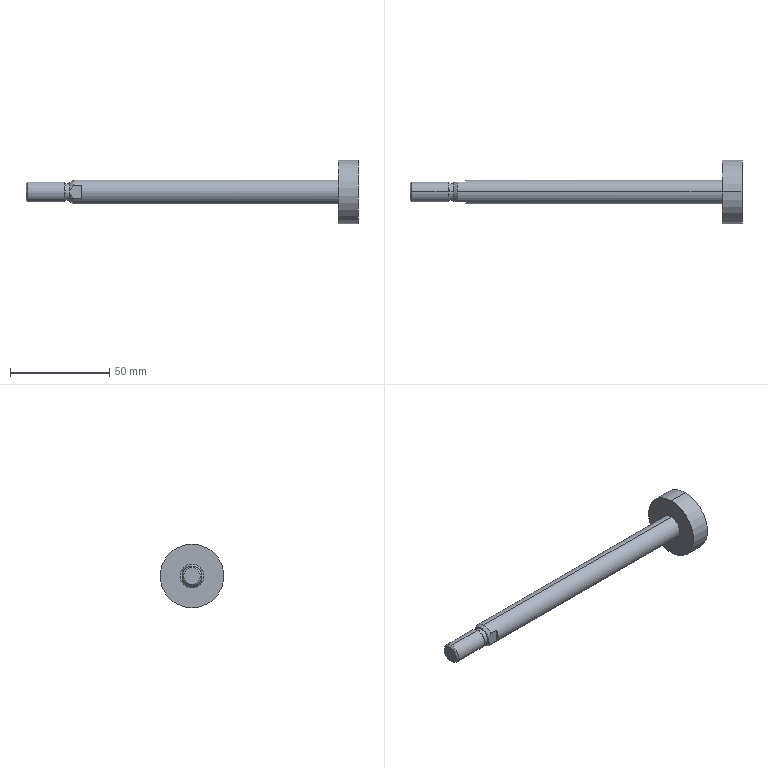Part | SolidWorks | features BaseBody 1 | 1 solid | 23 faces | box 166.9 x 32 x 32 mm | volume 24888 mm3 | plane 9 | cylinder 8 | cone 6 | commonest cylinder face diameters 8.4 x2 10 x2 12 x2 32 x2
STEP:
#1=CARTESIAN_POINT('',(-24.268,5.,3.317));
#2=VERTEX_POINT('',#1);
#3=CARTESIAN_POINT('',(-24.268,0.,6.));
#4=VERTEX_POINT('',#3);
#5=CARTESIAN_POINT('',(-24.268,0.,0.));
#6=DIRECTION('',(1.,0.,0.));
#7=DIRECTION('',(0.,0.,-1.));
#8=AXIS2_PLACEMENT_3D('',#5,#6,#7);
#9=CIRCLE('',#8,6.);
#10=EDGE_CURVE('',#2,#4,#9,.T.);
#11=ORIENTED_EDGE('',*,*,#10,.T.);
#12=CARTESIAN_POINT('',(108.9,0.,6.));
#13=VERTEX_POINT('',#12);
#14=CARTESIAN_POINT('',(118.9,0.,6.));
#15=DIRECTION('',(1.,0.,0.));
#16=VECTOR('',#15,1000.);
#17=LINE('',#14,#16);
#18=EDGE_CURVE('',#4,#13,#17,.T.);
#19=ORIENTED_EDGE('',*,*,#18,.T.);
#20=CARTESIAN_POINT('',(108.9,0.,-6.));
#21=VERTEX_POINT('',#20);
#22=CARTESIAN_POINT('',(108.9,0.,0.));
#23=DIRECTION('',(-1.,0.,0.));
#24=DIRECTION('',(0.,0.,-1.));
#25=AXIS2_PLACEMENT_3D('',#22,#23,#24);
#26=CIRCLE('',#25,6.);
#27=EDGE_CURVE('',#13,#21,#26,.T.);
#28=ORIENTED_EDGE('',*,*,#27,.T.);
#29=CARTESIAN_POINT('',(-24.268,0.,-6.));
#30=VERTEX_POINT('',#29);
#31=CARTESIAN_POINT('',(118.9,0.,-6.));
#32=DIRECTION('',(1.,0.,0.));
#33=VECTOR('',#32,1000.);
#34=LINE('',#31,#33);
#35=EDGE_CURVE('',#30,#21,#34,.T.);
#36=ORIENTED_EDGE('',*,*,#35,.F.);
#37=CARTESIAN_POINT('',(-24.268,5.,-3.317));
#38=VERTEX_POINT('',#37);
#39=CARTESIAN_POINT('',(-24.268,0.,0.));
#40=DIRECTION('',(1.,0.,0.));
#41=DIRECTION('',(0.,0.,-1.));
#42=AXIS2_PLACEMENT_3D('',#39,#40,#41);
#43=CIRCLE('',#42,6.);
#44=EDGE_CURVE('',#30,#38,#43,.T.);
#45=ORIENTED_EDGE('',*,*,#44,.T.);
#46=CARTESIAN_POINT('',(-20.,5.,-3.317));
#47=VERTEX_POINT('',#46);
#48=CARTESIAN_POINT('',(118.9,5.,-3.317));
#49=DIRECTION('',(1.,0.,0.));
#50=VECTOR('',#49,1000.);
#51=LINE('',#48,#50);
#52=EDGE_CURVE('',#38,#47,#51,.T.);
#53=ORIENTED_EDGE('',*,*,#52,.T.);
#54=CARTESIAN_POINT('',(-20.,5.,3.317));
#55=VERTEX_POINT('',#54);
#56=CARTESIAN_POINT('',(-20.,0.,0.));
#57=DIRECTION('',(1.,0.,0.));
#58=DIRECTION('',(0.,0.,-1.));
#59=AXIS2_PLACEMENT_3D('',#56,#57,#58);
#60=CIRCLE('',#59,6.);
#61=EDGE_CURVE('',#47,#55,#60,.T.);
#62=ORIENTED_EDGE('',*,*,#61,.T.);
#63=CARTESIAN_POINT('',(118.9,5.,3.317));
#64=DIRECTION('',(-1.,0.,0.));
#65=VECTOR('',#64,1000.);
#66=LINE('',#63,#65);
#67=EDGE_CURVE('',#55,#2,#66,.T.);
#68=ORIENTED_EDGE('',*,*,#67,.T.);
#69=EDGE_LOOP('',(#11,#19,#28,#36,#45,#53,#62,#68));
#70=FACE_OUTER_BOUND('',#69,.T.);
#71=CARTESIAN_POINT('',(118.9,0.,0.));
#72=DIRECTION('',(1.,0.,0.));
#73=DIRECTION('',(0.,0.,-1.));
#74=AXIS2_PLACEMENT_3D('',#71,#72,#73);
#75=CYLINDRICAL_SURFACE('',#74,6.);
#76=ADVANCED_FACE('',(#70),#75,.T.);
#77=CARTESIAN_POINT('',(108.9,0.,-16.));
#78=VERTEX_POINT('',#77);
#79=CARTESIAN_POINT('',(108.9,0.,16.));
#80=VERTEX_POINT('',#79);
#81=CARTESIAN_POINT('',(108.9,0.,0.));
#82=DIRECTION('',(1.,0.,0.));
#83=DIRECTION('',(0.,0.,-1.));
#84=AXIS2_PLACEMENT_3D('',#81,#82,#83);
#85=CIRCLE('',#84,16.);
#86=EDGE_CURVE('',#78,#80,#85,.T.);
#87=ORIENTED_EDGE('',*,*,#86,.T.);
#88=CARTESIAN_POINT('',(118.9,0.,16.));
#89=VERTEX_POINT('',#88);
#90=CARTESIAN_POINT('',(118.9,0.,16.));
#91=DIRECTION('',(1.,0.,0.));
#92=VECTOR('',#91,1000.);
#93=LINE('',#90,#92);
#94=EDGE_CURVE('',#80,#89,#93,.T.);
#95=ORIENTED_EDGE('',*,*,#94,.T.);
#96=CARTESIAN_POINT('',(118.9,0.,-16.));
#97=VERTEX_POINT('',#96);
#98=CARTESIAN_POINT('',(118.9,0.,0.));
#99=DIRECTION('',(-1.,0.,0.));
#100=DIRECTION('',(0.,0.,-1.));
#101=AXIS2_PLACEMENT_3D('',#98,#99,#100);
#102=CIRCLE('',#101,16.);
#103=EDGE_CURVE('',#89,#97,#102,.T.);
#104=ORIENTED_EDGE('',*,*,#103,.T.);
#105=CARTESIAN_POINT('',(118.9,0.,-16.));
#106=DIRECTION('',(1.,0.,0.));
#107=VECTOR('',#106,1000.);
#108=LINE('',#105,#107);
#109=EDGE_CURVE('',#78,#97,#108,.T.);
#110=ORIENTED_EDGE('',*,*,#109,.F.);
#111=EDGE_LOOP('',(#87,#95,#104,#110));
#112=FACE_OUTER_BOUND('',#111,.T.);
#113=CARTESIAN_POINT('',(118.9,0.,0.));
#114=DIRECTION('',(1.,0.,0.));
#115=DIRECTION('',(0.,0.,-1.));
#116=AXIS2_PLACEMENT_3D('',#113,#114,#115);
#117=CYLINDRICAL_SURFACE('',#116,16.);
#118=ADVANCED_FACE('',(#112),#117,.T.);
#119=CARTESIAN_POINT('',(-28.,0.,-4.2));
#120=VERTEX_POINT('',#119);
#121=CARTESIAN_POINT('',(-28.,0.,4.2));
#122=VERTEX_POINT('',#121);
#123=CARTESIAN_POINT('',(-28.,0.,0.));
#124=DIRECTION('',(1.,0.,0.));
#125=DIRECTION('',(0.,0.,-1.));
#126=AXIS2_PLACEMENT_3D('',#123,#124,#125);
#127=CIRCLE('',#126,4.2);
#128=EDGE_CURVE('',#120,#122,#127,.T.);
#129=ORIENTED_EDGE('',*,*,#128,.T.);
#130=CARTESIAN_POINT('',(-26.,0.,4.2));
#131=VERTEX_POINT('',#130);
#132=CARTESIAN_POINT('',(118.9,0.,4.2));
#133=DIRECTION('',(1.,0.,0.));
#134=VECTOR('',#133,1000.);
#135=LINE('',#132,#134);
#136=EDGE_CURVE('',#122,#131,#135,.T.);
#137=ORIENTED_EDGE('',*,*,#136,.T.);
#138=CARTESIAN_POINT('',(-26.,0.,-4.2));
#139=VERTEX_POINT('',#138);
#140=CARTESIAN_POINT('',(-26.,0.,0.));
#141=DIRECTION('',(-1.,0.,0.));
#142=DIRECTION('',(0.,0.,-1.));
#143=AXIS2_PLACEMENT_3D('',#140,#141,#142);
#144=CIRCLE('',#143,4.2);
#145=EDGE_CURVE('',#131,#139,#144,.T.);
#146=ORIENTED_EDGE('',*,*,#145,.T.);
#147=CARTESIAN_POINT('',(118.9,0.,-4.2));
#148=DIRECTION('',(1.,0.,0.));
#149=VECTOR('',#148,1000.);
#150=LINE('',#147,#149);
#151=EDGE_CURVE('',#120,#139,#150,.T.);
#152=ORIENTED_EDGE('',*,*,#151,.F.);
#153=EDGE_LOOP('',(#129,#137,#146,#152));
#154=FACE_OUTER_BOUND('',#153,.T.);
#155=CARTESIAN_POINT('',(118.9,0.,0.));
#156=DIRECTION('',(1.,0.,0.));
#157=DIRECTION('',(0.,0.,-1.));
#158=AXIS2_PLACEMENT_3D('',#155,#156,#157);
#159=CYLINDRICAL_SURFACE('',#158,4.2);
#160=ADVANCED_FACE('',(#154),#159,.T.);
#161=CARTESIAN_POINT('',(-28.,0.,4.233));
#162=VERTEX_POINT('',#161);
#163=CARTESIAN_POINT('',(-28.,0.,-4.233));
#164=VERTEX_POINT('',#163);
#165=CARTESIAN_POINT('',(-28.,0.,0.));
#166=DIRECTION('',(-1.,0.,0.));
#167=DIRECTION('',(0.,0.,1.));
#168=AXIS2_PLACEMENT_3D('',#165,#166,#167);
#169=CIRCLE('',#168,4.233);
#170=EDGE_CURVE('',#162,#164,#169,.T.);
#171=ORIENTED_EDGE('',*,*,#170,.T.);
#172=CARTESIAN_POINT('',(-28.767,0.,-5.));
#173=VERTEX_POINT('',#172);
#174=CARTESIAN_POINT('',(-28.767,0.,-5.));
#175=DIRECTION('',(-0.7071,0.,-0.7071));
#176=VECTOR('',#175,1000.);
#177=LINE('',#174,#176);
#178=EDGE_CURVE('',#164,#173,#177,.T.);
#179=ORIENTED_EDGE('',*,*,#178,.T.);
#180=CARTESIAN_POINT('',(-28.767,0.,5.));
#181=VERTEX_POINT('',#180);
#182=CARTESIAN_POINT('',(-28.767,0.,0.));
#183=DIRECTION('',(1.,0.,0.));
#184=DIRECTION('',(0.,0.,1.));
#185=AXIS2_PLACEMENT_3D('',#182,#183,#184);
#186=CIRCLE('',#185,5.);
#187=EDGE_CURVE('',#173,#181,#186,.T.);
#188=ORIENTED_EDGE('',*,*,#187,.T.);
#189=CARTESIAN_POINT('',(-28.767,0.,5.));
#190=DIRECTION('',(-0.7071,0.,0.7071));
#191=VECTOR('',#190,1000.);
#192=LINE('',#189,#191);
#193=EDGE_CURVE('',#162,#181,#192,.T.);
#194=ORIENTED_EDGE('',*,*,#193,.F.);
#195=EDGE_LOOP('',(#171,#179,#188,#194));
#196=FACE_OUTER_BOUND('',#195,.T.);
#197=CARTESIAN_POINT('',(-28.767,0.,0.));
#198=DIRECTION('',(-1.,0.,0.));
#199=DIRECTION('',(0.,0.,1.));
#200=AXIS2_PLACEMENT_3D('',#197,#198,#199);
#201=CONICAL_SURFACE('',#200,5.,0.7854);
#202=ADVANCED_FACE('',(#196),#201,.T.);
#203=CARTESIAN_POINT('',(-47.233,0.,-5.));
#204=VERTEX_POINT('',#203);
#205=CARTESIAN_POINT('',(-47.233,0.,5.));
#206=VERTEX_POINT('',#205);
#207=CARTESIAN_POINT('',(-47.233,0.,0.));
#208=DIRECTION('',(1.,0.,0.));
#209=DIRECTION('',(0.,0.,-1.));
#210=AXIS2_PLACEMENT_3D('',#207,#208,#209);
#211=CIRCLE('',#210,5.);
#212=EDGE_CURVE('',#204,#206,#211,.T.);
#213=ORIENTED_EDGE('',*,*,#212,.T.);
#214=CARTESIAN_POINT('',(118.9,0.,5.));
#215=DIRECTION('',(1.,0.,0.));
#216=VECTOR('',#215,1000.);
#217=LINE('',#214,#216);
#218=EDGE_CURVE('',#206,#181,#217,.T.);
#219=ORIENTED_EDGE('',*,*,#218,.T.);
#220=ORIENTED_EDGE('',*,*,#187,.F.);
#221=CARTESIAN_POINT('',(118.9,0.,-5.));
#222=DIRECTION('',(1.,0.,0.));
#223=VECTOR('',#222,1000.);
#224=LINE('',#221,#223);
#225=EDGE_CURVE('',#204,#173,#224,.T.);
#226=ORIENTED_EDGE('',*,*,#225,.F.);
#227=EDGE_LOOP('',(#213,#219,#220,#226));
#228=FACE_OUTER_BOUND('',#227,.T.);
#229=CARTESIAN_POINT('',(118.9,0.,0.));
#230=DIRECTION('',(1.,0.,0.));
#231=DIRECTION('',(0.,0.,-1.));
#232=AXIS2_PLACEMENT_3D('',#229,#230,#231);
#233=CYLINDRICAL_SURFACE('',#232,5.);
#234=ADVANCED_FACE('',(#228),#233,.T.);
#235=CARTESIAN_POINT('',(-48.,0.,-4.233));
#236=VERTEX_POINT('',#235);
#237=CARTESIAN_POINT('',(-48.,0.,4.233));
#238=VERTEX_POINT('',#237);
#239=CARTESIAN_POINT('',(-48.,0.,0.));
#240=DIRECTION('',(1.,0.,0.));
#241=DIRECTION('',(0.,0.,-1.));
#242=AXIS2_PLACEMENT_3D('',#239,#240,#241);
#243=CIRCLE('',#242,4.233);
#244=EDGE_CURVE('',#236,#238,#243,.T.);
#245=ORIENTED_EDGE('',*,*,#244,.T.);
#246=CARTESIAN_POINT('',(-47.233,0.,5.));
#247=DIRECTION('',(0.7071,0.,0.7071));
#248=VECTOR('',#247,1000.);
#249=LINE('',#246,#248);
#250=EDGE_CURVE('',#238,#206,#249,.T.);
#251=ORIENTED_EDGE('',*,*,#250,.T.);
#252=ORIENTED_EDGE('',*,*,#212,.F.);
#253=CARTESIAN_POINT('',(-47.233,0.,-5.));
#254=DIRECTION('',(0.7071,0.,-0.7071));
#255=VECTOR('',#254,1000.);
#256=LINE('',#253,#255);
#257=EDGE_CURVE('',#236,#204,#256,.T.);
#258=ORIENTED_EDGE('',*,*,#257,.F.);
#259=EDGE_LOOP('',(#245,#251,#252,#258));
#260=FACE_OUTER_BOUND('',#259,.T.);
#261=CARTESIAN_POINT('',(-47.233,0.,0.));
#262=DIRECTION('',(1.,0.,0.));
#263=DIRECTION('',(0.,0.,-1.));
#264=AXIS2_PLACEMENT_3D('',#261,#262,#263);
#265=CONICAL_SURFACE('',#264,5.,0.7854);
#266=ADVANCED_FACE('',(#260),#265,.T.);
#267=ORIENTED_EDGE('',*,*,#18,.F.);
#268=CARTESIAN_POINT('',(-24.268,-5.,3.317));
#269=VERTEX_POINT('',#268);
#270=CARTESIAN_POINT('',(-24.268,0.,0.));
#271=DIRECTION('',(1.,0.,0.));
#272=DIRECTION('',(0.,0.,-1.));
#273=AXIS2_PLACEMENT_3D('',#270,#271,#272);
#274=CIRCLE('',#273,6.);
#275=EDGE_CURVE('',#4,#269,#274,.T.);
#276=ORIENTED_EDGE('',*,*,#275,.T.);
#277=CARTESIAN_POINT('',(-20.,-5.,3.317));
#278=VERTEX_POINT('',#277);
#279=CARTESIAN_POINT('',(118.9,-5.,3.317));
#280=DIRECTION('',(1.,0.,0.));
#281=VECTOR('',#280,1000.);
#282=LINE('',#279,#281);
#283=EDGE_CURVE('',#269,#278,#282,.T.);
#284=ORIENTED_EDGE('',*,*,#283,.T.);
#285=CARTESIAN_POINT('',(-20.,-5.,-3.317));
#286=VERTEX_POINT('',#285);
#287=CARTESIAN_POINT('',(-20.,0.,0.));
#288=DIRECTION('',(1.,0.,0.));
#289=DIRECTION('',(0.,0.,-1.));
#290=AXIS2_PLACEMENT_3D('',#287,#288,#289);
#291=CIRCLE('',#290,6.);
#292=EDGE_CURVE('',#278,#286,#291,.T.);
#293=ORIENTED_EDGE('',*,*,#292,.T.);
#294=CARTESIAN_POINT('',(-24.268,-5.,-3.317));
#295=VERTEX_POINT('',#294);
#296=CARTESIAN_POINT('',(118.9,-5.,-3.317));
#297=DIRECTION('',(-1.,0.,0.));
#298=VECTOR('',#297,1000.);
#299=LINE('',#296,#298);
#300=EDGE_CURVE('',#286,#295,#299,.T.);
#301=ORIENTED_EDGE('',*,*,#300,.T.);
#302=CARTESIAN_POINT('',(-24.268,0.,0.));
#303=DIRECTION('',(1.,0.,0.));
#304=DIRECTION('',(0.,0.,-1.));
#305=AXIS2_PLACEMENT_3D('',#302,#303,#304);
#306=CIRCLE('',#305,6.);
#307=EDGE_CURVE('',#295,#30,#306,.T.);
#308=ORIENTED_EDGE('',*,*,#307,.T.);
#309=ORIENTED_EDGE('',*,*,#35,.T.);
#310=CARTESIAN_POINT('',(108.9,0.,0.));
#311=DIRECTION('',(-1.,0.,0.));
#312=DIRECTION('',(0.,0.,-1.));
#313=AXIS2_PLACEMENT_3D('',#310,#311,#312);
#314=CIRCLE('',#313,6.);
#315=EDGE_CURVE('',#21,#13,#314,.T.);
#316=ORIENTED_EDGE('',*,*,#315,.T.);
#317=EDGE_LOOP('',(#267,#276,#284,#293,#301,#308,#309,#316));
#318=FACE_OUTER_BOUND('',#317,.T.);
#319=CARTESIAN_POINT('',(118.9,0.,0.));
#320=DIRECTION('',(1.,0.,0.));
#321=DIRECTION('',(0.,0.,-1.));
#322=AXIS2_PLACEMENT_3D('',#319,#320,#321);
#323=CYLINDRICAL_SURFACE('',#322,6.);
#324=ADVANCED_FACE('',(#318),#323,.T.);
#325=ORIENTED_EDGE('',*,*,#315,.F.);
#326=ORIENTED_EDGE('',*,*,#27,.F.);
#327=EDGE_LOOP('',(#325,#326));
#328=FACE_BOUND('',#327,.T.);
#329=ORIENTED_EDGE('',*,*,#86,.F.);
#330=CARTESIAN_POINT('',(108.9,0.,0.));
#331=DIRECTION('',(1.,0.,0.));
#332=DIRECTION('',(0.,0.,-1.));
#333=AXIS2_PLACEMENT_3D('',#330,#331,#332);
#334=CIRCLE('',#333,16.);
#335=EDGE_CURVE('',#80,#78,#334,.T.);
#336=ORIENTED_EDGE('',*,*,#335,.F.);
#337=EDGE_LOOP('',(#329,#336));
#338=FACE_OUTER_BOUND('',#337,.T.);
#339=CARTESIAN_POINT('',(108.9,6.,0.));
#340=DIRECTION('',(1.,0.,0.));
#341=DIRECTION('',(0.,0.,-1.));
#342=AXIS2_PLACEMENT_3D('',#339,#340,#341);
#343=PLANE('',#342);
#344=ADVANCED_FACE('',(#328,#338),#343,.F.);
#345=CARTESIAN_POINT('',(-26.,-5.,0.));
#346=VERTEX_POINT('',#345);
#347=CARTESIAN_POINT('',(-24.268,-5.,-3.317));
#348=CARTESIAN_POINT('',(-24.489,-5.,-3.086));
#349=CARTESIAN_POINT('',(-24.701,-5.,-2.848));
#350=CARTESIAN_POINT('',(-25.098,-5.,-2.352));
#351=CARTESIAN_POINT('',(-25.282,-5.,-2.093));
#352=CARTESIAN_POINT('',(-25.608,-5.,-1.544));
#353=CARTESIAN_POINT('',(-25.748,-5.,-1.251));
#354=CARTESIAN_POINT('',(-25.944,-5.,-0.6446));
#355=CARTESIAN_POINT('',(-26.,-5.,-0.3234));
#356=CARTESIAN_POINT('',(-26.,-5.,0.));
#357=B_SPLINE_CURVE_WITH_KNOTS('',3,(#347,#348,#349,#350,#351,#352,#353,#354,#355,#356),.UNSPECIFIED.,.F.,.F.,(4,2,2,2,4),(0.,0.0009524,0.001905,0.002857,0.00381),.UNSPECIFIED.);
#358=EDGE_CURVE('',#295,#346,#357,.T.);
#359=ORIENTED_EDGE('',*,*,#358,.F.);
#360=ORIENTED_EDGE('',*,*,#300,.F.);
#361=CARTESIAN_POINT('',(-20.,-5.,8.));
#362=DIRECTION('',(0.,0.,-1.));
#363=VECTOR('',#362,1000.);
#364=LINE('',#361,#363);
#365=EDGE_CURVE('',#278,#286,#364,.T.);
#366=ORIENTED_EDGE('',*,*,#365,.F.);
#367=ORIENTED_EDGE('',*,*,#283,.F.);
#368=CARTESIAN_POINT('',(-26.,-5.,0.));
#369=CARTESIAN_POINT('',(-26.,-5.,0.3237));
#370=CARTESIAN_POINT('',(-25.945,-5.,0.6366));
#371=CARTESIAN_POINT('',(-25.799,-5.,1.093));
#372=CARTESIAN_POINT('',(-25.739,-5.,1.244));
#373=CARTESIAN_POINT('',(-25.605,-5.,1.534));
#374=CARTESIAN_POINT('',(-25.53,-5.,1.674));
#375=CARTESIAN_POINT('',(-25.288,-5.,2.085));
#376=CARTESIAN_POINT('',(-25.103,-5.,2.345));
#377=CARTESIAN_POINT('',(-24.703,-5.,2.846));
#378=CARTESIAN_POINT('',(-24.49,-5.,3.085));
#379=CARTESIAN_POINT('',(-24.268,-5.,3.317));
#380=B_SPLINE_CURVE_WITH_KNOTS('',3,(#368,#369,#370,#371,#372,#373,#374,#375,#376,#377,#378,#379),.UNSPECIFIED.,.F.,.F.,(4,2,2,2,2,4),(0.,0.0009528,0.001429,0.001906,0.002858,0.003811),.UNSPECIFIED.);
#381=EDGE_CURVE('',#346,#269,#380,.T.);
#382=ORIENTED_EDGE('',*,*,#381,.F.);
#383=EDGE_LOOP('',(#359,#360,#366,#367,#382));
#384=FACE_OUTER_BOUND('',#383,.T.);
#385=CARTESIAN_POINT('',(-20.,-5.,8.));
#386=DIRECTION('',(0.,1.,0.));
#387=DIRECTION('',(0.,0.,1.));
#388=AXIS2_PLACEMENT_3D('',#385,#386,#387);
#389=PLANE('',#388);
#390=ADVANCED_FACE('',(#384),#389,.F.);
#391=ORIENTED_EDGE('',*,*,#292,.F.);
#392=ORIENTED_EDGE('',*,*,#365,.T.);
#393=EDGE_LOOP('',(#391,#392));
#394=FACE_OUTER_BOUND('',#393,.T.);
#395=CARTESIAN_POINT('',(-20.,0.,0.));
#396=DIRECTION('',(1.,0.,0.));
#397=DIRECTION('',(0.,0.,-1.));
#398=AXIS2_PLACEMENT_3D('',#395,#396,#397);
#399=PLANE('',#398);
#400=ADVANCED_FACE('',(#394),#399,.F.);
#401=CARTESIAN_POINT('',(-26.,5.,0.));
#402=VERTEX_POINT('',#401);
#403=CARTESIAN_POINT('',(-26.,0.,0.));
#404=DIRECTION('',(1.,0.,0.));
#405=DIRECTION('',(0.,1.,0.));
#406=AXIS2_PLACEMENT_3D('',#403,#404,#405);
#407=CIRCLE('',#406,5.);
#408=EDGE_CURVE('',#402,#346,#407,.T.);
#409=ORIENTED_EDGE('',*,*,#408,.T.);
#410=ORIENTED_EDGE('',*,*,#381,.T.);
#411=ORIENTED_EDGE('',*,*,#275,.F.);
#412=ORIENTED_EDGE('',*,*,#10,.F.);
#413=CARTESIAN_POINT('',(-24.268,5.,3.317));
#414=CARTESIAN_POINT('',(-24.489,5.,3.086));
#415=CARTESIAN_POINT('',(-24.701,5.,2.848));
#416=CARTESIAN_POINT('',(-25.098,5.,2.352));
#417=CARTESIAN_POINT('',(-25.282,5.,2.093));
#418=CARTESIAN_POINT('',(-25.608,5.,1.544));
#419=CARTESIAN_POINT('',(-25.748,5.,1.251));
#420=CARTESIAN_POINT('',(-25.944,5.,0.6446));
#421=CARTESIAN_POINT('',(-26.,5.,0.3234));
#422=CARTESIAN_POINT('',(-26.,5.,0.));
#423=B_SPLINE_CURVE_WITH_KNOTS('',3,(#413,#414,#415,#416,#417,#418,#419,#420,#421,#422),.UNSPECIFIED.,.F.,.F.,(4,2,2,2,4),(0.,0.0009524,0.001905,0.002857,0.00381),.UNSPECIFIED.);
#424=EDGE_CURVE('',#2,#402,#423,.T.);
#425=ORIENTED_EDGE('',*,*,#424,.T.);
#426=EDGE_LOOP('',(#409,#410,#411,#412,#425));
#427=FACE_OUTER_BOUND('',#426,.T.);
#428=CARTESIAN_POINT('',(-24.268,0.,0.));
#429=DIRECTION('',(1.,0.,0.));
#430=DIRECTION('',(0.,1.,0.));
#431=AXIS2_PLACEMENT_3D('',#428,#429,#430);
#432=CONICAL_SURFACE('',#431,6.,0.5236);
#433=ADVANCED_FACE('',(#427),#432,.T.);
#434=ORIENTED_EDGE('',*,*,#424,.F.);
#435=ORIENTED_EDGE('',*,*,#67,.F.);
#436=CARTESIAN_POINT('',(-20.,5.,-8.));
#437=DIRECTION('',(0.,0.,1.));
#438=VECTOR('',#437,1000.);
#439=LINE('',#436,#438);
#440=EDGE_CURVE('',#47,#55,#439,.T.);
#441=ORIENTED_EDGE('',*,*,#440,.F.);
#442=ORIENTED_EDGE('',*,*,#52,.F.);
#443=CARTESIAN_POINT('',(-26.,5.,0.));
#444=CARTESIAN_POINT('',(-26.,5.,-0.3237));
#445=CARTESIAN_POINT('',(-25.945,5.,-0.6366));
#446=CARTESIAN_POINT('',(-25.799,5.,-1.093));
#447=CARTESIAN_POINT('',(-25.739,5.,-1.244));
#448=CARTESIAN_POINT('',(-25.605,5.,-1.534));
#449=CARTESIAN_POINT('',(-25.53,5.,-1.674));
#450=CARTESIAN_POINT('',(-25.288,5.,-2.085));
#451=CARTESIAN_POINT('',(-25.103,5.,-2.345));
#452=CARTESIAN_POINT('',(-24.703,5.,-2.846));
#453=CARTESIAN_POINT('',(-24.49,5.,-3.085));
#454=CARTESIAN_POINT('',(-24.268,5.,-3.317));
#455=B_SPLINE_CURVE_WITH_KNOTS('',3,(#443,#444,#445,#446,#447,#448,#449,#450,#451,#452,#453,#454),.UNSPECIFIED.,.F.,.F.,(4,2,2,2,2,4),(0.,0.0009528,0.001429,0.001906,0.002858,0.003811),.UNSPECIFIED.);
#456=EDGE_CURVE('',#402,#38,#455,.T.);
#457=ORIENTED_EDGE('',*,*,#456,.F.);
#458=EDGE_LOOP('',(#434,#435,#441,#442,#457));
#459=FACE_OUTER_BOUND('',#458,.T.);
#460=CARTESIAN_POINT('',(-20.,5.,-8.));
#461=DIRECTION('',(0.,-1.,0.));
#462=DIRECTION('',(0.,0.,-1.));
#463=AXIS2_PLACEMENT_3D('',#460,#461,#462);
#464=PLANE('',#463);
#465=ADVANCED_FACE('',(#459),#464,.F.);
#466=ORIENTED_EDGE('',*,*,#61,.F.);
#467=ORIENTED_EDGE('',*,*,#440,.T.);
#468=EDGE_LOOP('',(#466,#467));
#469=FACE_OUTER_BOUND('',#468,.T.);
#470=CARTESIAN_POINT('',(-20.,0.,0.));
#471=DIRECTION('',(1.,0.,0.));
#472=DIRECTION('',(0.,0.,-1.));
#473=AXIS2_PLACEMENT_3D('',#470,#471,#472);
#474=PLANE('',#473);
#475=ADVANCED_FACE('',(#469),#474,.F.);
#476=ORIENTED_EDGE('',*,*,#307,.F.);
#477=ORIENTED_EDGE('',*,*,#358,.T.);
#478=CARTESIAN_POINT('',(-26.,0.,0.));
#479=DIRECTION('',(1.,0.,0.));
#480=DIRECTION('',(0.,1.,0.));
#481=AXIS2_PLACEMENT_3D('',#478,#479,#480);
#482=CIRCLE('',#481,5.);
#483=EDGE_CURVE('',#346,#402,#482,.T.);
#484=ORIENTED_EDGE('',*,*,#483,.T.);
#485=ORIENTED_EDGE('',*,*,#456,.T.);
#486=ORIENTED_EDGE('',*,*,#44,.F.);
#487=EDGE_LOOP('',(#476,#477,#484,#485,#486));
#488=FACE_OUTER_BOUND('',#487,.T.);
#489=CARTESIAN_POINT('',(-24.268,0.,0.));
#490=DIRECTION('',(1.,0.,0.));
#491=DIRECTION('',(0.,1.,0.));
#492=AXIS2_PLACEMENT_3D('',#489,#490,#491);
#493=CONICAL_SURFACE('',#492,6.,0.5236);
#494=ADVANCED_FACE('',(#488),#493,.T.);
#495=ORIENTED_EDGE('',*,*,#94,.F.);
#496=ORIENTED_EDGE('',*,*,#335,.T.);
#497=ORIENTED_EDGE('',*,*,#109,.T.);
#498=CARTESIAN_POINT('',(118.9,0.,0.));
#499=DIRECTION('',(-1.,0.,0.));
#500=DIRECTION('',(0.,0.,-1.));
#501=AXIS2_PLACEMENT_3D('',#498,#499,#500);
#502=CIRCLE('',#501,16.);
#503=EDGE_CURVE('',#97,#89,#502,.T.);
#504=ORIENTED_EDGE('',*,*,#503,.T.);
#505=EDGE_LOOP('',(#495,#496,#497,#504));
#506=FACE_OUTER_BOUND('',#505,.T.);
#507=CARTESIAN_POINT('',(118.9,0.,0.));
#508=DIRECTION('',(1.,0.,0.));
#509=DIRECTION('',(0.,0.,-1.));
#510=AXIS2_PLACEMENT_3D('',#507,#508,#509);
#511=CYLINDRICAL_SURFACE('',#510,16.);
#512=ADVANCED_FACE('',(#506),#511,.T.);
#513=CARTESIAN_POINT('',(-26.,0.,0.));
#514=DIRECTION('',(-1.,0.,0.));
#515=DIRECTION('',(0.,0.,-1.));
#516=AXIS2_PLACEMENT_3D('',#513,#514,#515);
#517=CIRCLE('',#516,4.2);
#518=EDGE_CURVE('',#139,#131,#517,.T.);
#519=ORIENTED_EDGE('',*,*,#518,.F.);
#520=ORIENTED_EDGE('',*,*,#145,.F.);
#521=EDGE_LOOP('',(#519,#520));
#522=FACE_BOUND('',#521,.T.);
#523=ORIENTED_EDGE('',*,*,#483,.F.);
#524=ORIENTED_EDGE('',*,*,#408,.F.);
#525=EDGE_LOOP('',(#523,#524));
#526=FACE_OUTER_BOUND('',#525,.T.);
#527=CARTESIAN_POINT('',(-26.,4.2,0.));
#528=DIRECTION('',(1.,0.,0.));
#529=DIRECTION('',(0.,0.,-1.));
#530=AXIS2_PLACEMENT_3D('',#527,#528,#529);
#531=PLANE('',#530);
#532=ADVANCED_FACE('',(#522,#526),#531,.F.);
#533=ORIENTED_EDGE('',*,*,#503,.F.);
#534=ORIENTED_EDGE('',*,*,#103,.F.);
#535=EDGE_LOOP('',(#533,#534));
#536=FACE_OUTER_BOUND('',#535,.T.);
#537=CARTESIAN_POINT('',(118.9,16.,0.));
#538=DIRECTION('',(-1.,0.,0.));
#539=DIRECTION('',(0.,0.,1.));
#540=AXIS2_PLACEMENT_3D('',#537,#538,#539);
#541=PLANE('',#540);
#542=ADVANCED_FACE('',(#536),#541,.F.);
#543=ORIENTED_EDGE('',*,*,#136,.F.);
#544=CARTESIAN_POINT('',(-28.,0.,0.));
#545=DIRECTION('',(1.,0.,0.));
#546=DIRECTION('',(0.,0.,-1.));
#547=AXIS2_PLACEMENT_3D('',#544,#545,#546);
#548=CIRCLE('',#547,4.2);
#549=EDGE_CURVE('',#122,#120,#548,.T.);
#550=ORIENTED_EDGE('',*,*,#549,.T.);
#551=ORIENTED_EDGE('',*,*,#151,.T.);
#552=ORIENTED_EDGE('',*,*,#518,.T.);
#553=EDGE_LOOP('',(#543,#550,#551,#552));
#554=FACE_OUTER_BOUND('',#553,.T.);
#555=CARTESIAN_POINT('',(118.9,0.,0.));
#556=DIRECTION('',(1.,0.,0.));
#557=DIRECTION('',(0.,0.,-1.));
#558=AXIS2_PLACEMENT_3D('',#555,#556,#557);
#559=CYLINDRICAL_SURFACE('',#558,4.2);
#560=ADVANCED_FACE('',(#554),#559,.T.);
#561=ORIENTED_EDGE('',*,*,#170,.F.);
#562=CARTESIAN_POINT('',(-28.,0.,0.));
#563=DIRECTION('',(-1.,0.,0.));
#564=DIRECTION('',(0.,0.,1.));
#565=AXIS2_PLACEMENT_3D('',#562,#563,#564);
#566=CIRCLE('',#565,4.233);
#567=EDGE_CURVE('',#164,#162,#566,.T.);
#568=ORIENTED_EDGE('',*,*,#567,.F.);
#569=EDGE_LOOP('',(#561,#568));
#570=FACE_OUTER_BOUND('',#569,.T.);
#571=ORIENTED_EDGE('',*,*,#128,.F.);
#572=ORIENTED_EDGE('',*,*,#549,.F.);
#573=EDGE_LOOP('',(#571,#572));
#574=FACE_BOUND('',#573,.T.);
#575=CARTESIAN_POINT('',(-28.,4.233,0.));
#576=DIRECTION('',(-1.,0.,0.));
#577=DIRECTION('',(0.,0.,1.));
#578=AXIS2_PLACEMENT_3D('',#575,#576,#577);
#579=PLANE('',#578);
#580=ADVANCED_FACE('',(#570,#574),#579,.F.);
#581=ORIENTED_EDGE('',*,*,#178,.F.);
#582=ORIENTED_EDGE('',*,*,#567,.T.);
#583=ORIENTED_EDGE('',*,*,#193,.T.);
#584=CARTESIAN_POINT('',(-28.767,0.,0.));
#585=DIRECTION('',(1.,0.,0.));
#586=DIRECTION('',(0.,0.,1.));
#587=AXIS2_PLACEMENT_3D('',#584,#585,#586);
#588=CIRCLE('',#587,5.);
#589=EDGE_CURVE('',#181,#173,#588,.T.);
#590=ORIENTED_EDGE('',*,*,#589,.T.);
#591=EDGE_LOOP('',(#581,#582,#583,#590));
#592=FACE_OUTER_BOUND('',#591,.T.);
#593=CARTESIAN_POINT('',(-28.767,0.,0.));
#594=DIRECTION('',(-1.,0.,0.));
#595=DIRECTION('',(0.,0.,1.));
#596=AXIS2_PLACEMENT_3D('',#593,#594,#595);
#597=CONICAL_SURFACE('',#596,5.,0.7854);
#598=ADVANCED_FACE('',(#592),#597,.T.);
#599=ORIENTED_EDGE('',*,*,#218,.F.);
#600=CARTESIAN_POINT('',(-47.233,0.,0.));
#601=DIRECTION('',(1.,0.,0.));
#602=DIRECTION('',(0.,0.,-1.));
#603=AXIS2_PLACEMENT_3D('',#600,#601,#602);
#604=CIRCLE('',#603,5.);
#605=EDGE_CURVE('',#206,#204,#604,.T.);
#606=ORIENTED_EDGE('',*,*,#605,.T.);
#607=ORIENTED_EDGE('',*,*,#225,.T.);
#608=ORIENTED_EDGE('',*,*,#589,.F.);
#609=EDGE_LOOP('',(#599,#606,#607,#608));
#610=FACE_OUTER_BOUND('',#609,.T.);
#611=CARTESIAN_POINT('',(118.9,0.,0.));
#612=DIRECTION('',(1.,0.,0.));
#613=DIRECTION('',(0.,0.,-1.));
#614=AXIS2_PLACEMENT_3D('',#611,#612,#613);
#615=CYLINDRICAL_SURFACE('',#614,5.);
#616=ADVANCED_FACE('',(#610),#615,.T.);
#617=ORIENTED_EDGE('',*,*,#250,.F.);
#618=CARTESIAN_POINT('',(-48.,0.,0.));
#619=DIRECTION('',(1.,0.,0.));
#620=DIRECTION('',(0.,0.,-1.));
#621=AXIS2_PLACEMENT_3D('',#618,#619,#620);
#622=CIRCLE('',#621,4.233);
#623=EDGE_CURVE('',#238,#236,#622,.T.);
#624=ORIENTED_EDGE('',*,*,#623,.T.);
#625=ORIENTED_EDGE('',*,*,#257,.T.);
#626=ORIENTED_EDGE('',*,*,#605,.F.);
#627=EDGE_LOOP('',(#617,#624,#625,#626));
#628=FACE_OUTER_BOUND('',#627,.T.);
#629=CARTESIAN_POINT('',(-47.233,0.,0.));
#630=DIRECTION('',(1.,0.,0.));
#631=DIRECTION('',(0.,0.,-1.));
#632=AXIS2_PLACEMENT_3D('',#629,#630,#631);
#633=CONICAL_SURFACE('',#632,5.,0.7854);
#634=ADVANCED_FACE('',(#628),#633,.T.);
#635=ORIENTED_EDGE('',*,*,#244,.F.);
#636=ORIENTED_EDGE('',*,*,#623,.F.);
#637=EDGE_LOOP('',(#635,#636));
#638=FACE_OUTER_BOUND('',#637,.T.);
#639=CARTESIAN_POINT('',(-48.,0.,0.));
#640=DIRECTION('',(1.,0.,0.));
#641=DIRECTION('',(0.,0.,-1.));
#642=AXIS2_PLACEMENT_3D('',#639,#640,#641);
#643=PLANE('',#642);
#644=ADVANCED_FACE('',(#638),#643,.F.);
#645=CLOSED_SHELL('',(#76,#118,#160,#202,#234,#266,#324,#344,#390,#400,#433,#465,#475,#494,#512,#532,#542,#560,#580,#598,#616,#634,#644));
#646=MANIFOLD_SOLID_BREP('',#645);
#647=CARTESIAN_POINT('',(0.,0.,0.));
#648=DIRECTION('',(0.,0.,1.));
#649=DIRECTION('',(1.,0.,0.));
#650=AXIS2_PLACEMENT_3D('',#647,#648,#649);
#651=(LENGTH_UNIT()NAMED_UNIT(*)SI_UNIT(.MILLI.,.METRE.));
#652=UNCERTAINTY_MEASURE_WITH_UNIT(LENGTH_MEASURE(0.00001),#651,'','');
#653=(NAMED_UNIT(*)PLANE_ANGLE_UNIT()SI_UNIT($,.RADIAN.));
#654=(NAMED_UNIT(*)SI_UNIT($,.STERADIAN.)SOLID_ANGLE_UNIT());
#655=(GEOMETRIC_REPRESENTATION_CONTEXT(3)GLOBAL_UNCERTAINTY_ASSIGNED_CONTEXT((#652))GLOBAL_UNIT_ASSIGNED_CONTEXT((#651,#653,#654))REPRESENTATION_CONTEXT('',''));
#656=ADVANCED_BREP_SHAPE_REPRESENTATION('',(#646,#650),#655);